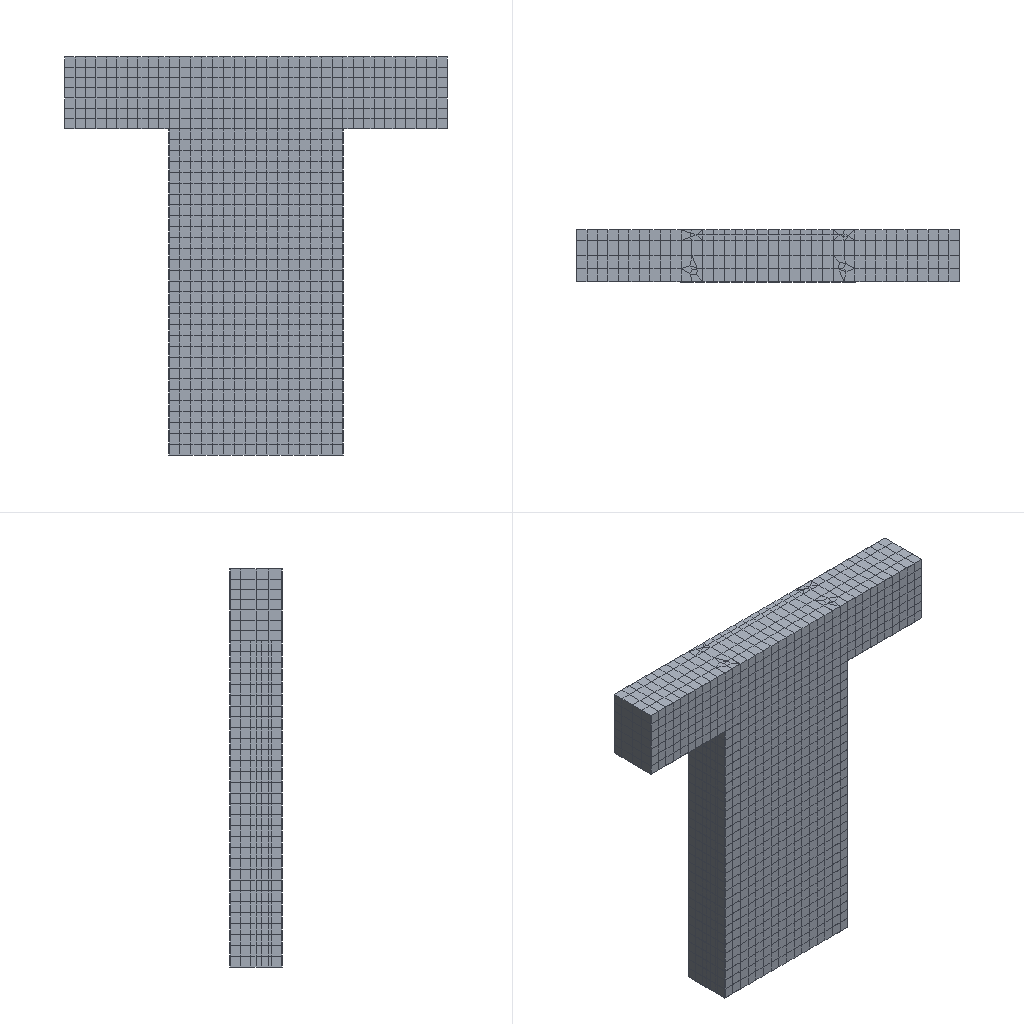Simulation study | abaqus
Set-up summary:
category,name,step,type,value,unit,region
solver,abaqus
solver,version,,,Abaqus/Standard 2020
units,not stated in the deck,,not stated
analysis,deck,,static,static
load_step,Step-1,Step-1,static
load_step,Step-2,Step-2,static
load_step,requested,,,2
mesh,nodes,,,10068
mesh,elements,,,7418
element_type,C3D6,,solid,444
element_type,T3D2,,truss,2018
element_type,C3D8R,,solid,4956
load,load commands in deck,,count,2
bc,support commands in deck,,count,7
material,CON,,in results
material,Q235,,in results
check,setup vs results,,match,"per instance, exact: element labels, types and connectivity; labels of the nodes the elements use; coordinates of those nodes at SINGLE_PRECISION in 1 of 4 instance(s)"
Abaqus input file, long lists of numbers shortened:
*Heading
** Job name: Job-3 Model name: Model-1-Copy-Copy
** Generated by: Abaqus/CAE 2020
*Preprint, echo=NO, model=NO, history=NO, contact=NO
**
** PARTS
**
*Part, name=con
*Node
      1,         489.,          90.,        1500.
      2,        -111.,          90.,        1500.
** (5932 more lines like these left out)
*Element, type=C3D8R
  1,    5, 1585,  129,    1, 1654, 3925, 3903, 1653
  2, 1585, 1586,  130,  129, 3925, 3926, 3904, 3903
** (3814 more lines like these left out)
*Element, type=C3D6
1093,    5,   23,    1,  345,  546,  307
1094, 2438,   27,   28, 4466,  439,  547
** (442 more lines like these left out)
*Nset, nset=Set-12
    1,    2,    3,    4,    5,    6,    7,    8,    9,   10,   11,   12,   13,   14,   15,   16
   17,   18,   19,   20,   21,   22,   23,   24,   25,   26,   27,   28,   29,   30,   31,   32
** (360 more lines like these left out)
*Elset, elset=Set-12
    1,    2,    3,    4,    5,    6,    7,    8,    9,   10,   11,   12,   13,   14,   15,   16
   17,   18,   19,   20,   21,   22,   23,   24,   25,   26,   27,   28,   29,   30,   31,   32
** (249 more lines like these left out)
*Nset, nset=Set-14, generate
    1,  5934,     1
*Elset, elset=Set-14, generate
    1,  4260,     1
** Section: con
*Solid Section, elset=Set-14, material=con
,
*End Part
**
*Part, name=fiber
*Node
      1,         734.,          52.,        1525.
      2,         734.,         115.,        1525.
** (1652 more lines like these left out)
*Element, type=T3D2
1, 2, 1
2,   3, 873
** (2016 more lines like these left out)
*Nset, nset=Set-3, generate
    1,  1654,     1
*Elset, elset=Set-3, generate
    1,  2018,     1
*Nset, nset=nei
    1,    2,    3,    4,    5,    6,    7,    8,    9,   10,   11,   12,   13,   14,   15,   16
   17,   18,   19,   20,   21,   22,   23,   24,   25,   26,   27,   28,   29,   30,   31,   32
** (39 more lines like these left out)
*Elset, elset=nei
    1,    2,    3,    4,    5,    6,    7,    8,    9,   10,   11,   12,   13,   14,   15,   16
   17,   18,   19,   20,   21,   22,   23,   24,   25,   26,   27,   28,   29,   30,   31,   32
** (45 more lines like these left out)
** Section: fiber
*Solid Section, elset=Set-3, material=q235
12.56,
*End Part
**
*Part, name=liang1
*Node
      1,         588.,         140.,        1500.
      2,         588.,         140.,           0.
** (1238 more lines like these left out)
*Element, type=C3D8R
 1,   8, 145, 922, 176,   1,  57, 893, 116
 2, 145, 144, 923, 922,  57,  58, 894, 893
** (568 more lines like these left out)
*Nset, nset=Set-1, generate
    1,  1240,     1
*Elset, elset=Set-1, generate
   1,  570,    1
** Section: liang
*Solid Section, elset=Set-1, material=q235
,
*End Part
**
*Part, name=liang2
*Node
      1,        -112.,         -99.,           0.
      2,        -112.,         -99.,        1500.
** (1238 more lines like these left out)
*Element, type=C3D8R
 1, 174, 893, 922, 173,   1,  57, 114,   4
 2, 893, 894, 923, 922,  57,  58, 113, 114
** (568 more lines like these left out)
*Nset, nset=Set-1, generate
    1,  1240,     1
*Elset, elset=Set-1, generate
   1,  570,    1
** Section: liang
*Solid Section, elset=Set-1, material=q235
,
*End Part
**
**
** ASSEMBLY
**
*Assembly, name=Assembly
**
*Instance, name=con-1, part=con
*End Instance
**
*Instance, name=fiber-1, part=fiber
*End Instance
**
*Instance, name=liang1-1, part=liang1
*End Instance
**
*Instance, name=liang2-1, part=liang2
*End Instance
**
*Node
      1,         189.,          20.,           0.
*Node
      2,         189.,          20.,        1830.
*Nset, nset=Set-15
 1,
*Nset, nset=Set-16
 1,
*Nset, nset=Set-18
 2,
*Nset, nset=insert, instance=fiber-1
    1,    2,    3,    4,    5,    6,    7,    8,    9,   10,   11,   12,   13,   14,   15,   16
   17,   18,   19,   20,   21,   22,   23,   24,   25,   26,   27,   28,   29,   30,   31,   32
** (42 more lines like these left out)
*Nset, nset=m_Set-6, instance=fiber-1
    1,    2,    3,    4,    5,    6,    7,    8,    9,   10,   11,   12,   13,   14,   15,   16
   17,   18,   19,   20,   21,   22,   23,   24,   25,   26,   27,   28,   29,   30,   31,   32
** (40 more lines like these left out)
*Elset, elset=m_Set-6, instance=fiber-1
    1,    2,    3,    4,    5,    6,    7,    8,    9,   10,   11,   12,   13,   14,   15,   16
   17,   18,   19,   20,   21,   22,   23,   24,   25,   26,   27,   28,   29,   30,   31,   32
** (48 more lines like these left out)
*Nset, nset=m_Set-8, instance=fiber-1
    1,    2,    3,    4,    5,    6,    7,    8,    9,   10,   11,   12,   13,   14,   15,   16
   17,   18,   19,   20,   21,   22,   23,   24,   25,   26,   27,   28,   29,   30,   31,   32
** (38 more lines like these left out)
*Elset, elset=m_Set-8, instance=fiber-1
    1,    2,    3,    4,    5,    6,    7,    8,    9,   10,   11,   12,   13,   14,   15,   16
   17,   18,   19,   20,   21,   22,   23,   24,   25,   26,   27,   28,   29,   30,   31,   32
** (45 more lines like these left out)
*Nset, nset=m_Set-10, instance=fiber-1
    1,    2,    3,    4,    5,    6,    7,    8,    9,   10,   11,   12,   13,   14,   15,   16
   17,   18,   19,   20,   21,   22,   23,   24,   25,   26,   27,   28,   29,   30,   31,   32
** (38 more lines like these left out)
*Elset, elset=m_Set-10, instance=fiber-1
    1,    2,    3,    4,    5,    6,    7,    8,    9,   10,   11,   12,   13,   14,   15,   16
   17,   18,   19,   20,   21,   22,   23,   24,   25,   26,   27,   28,   29,   30,   31,   32
** (45 more lines like these left out)
*Nset, nset=m_Set-12, instance=fiber-1
    1,    2,    3,    4,    5,    6,    7,    8,    9,   10,   11,   12,   13,   14,   15,   16
   17,   18,   19,   20,   21,   22,   23,   24,   25,   26,   27,   28,   29,   30,   31,   32
** (91 more lines like these left out)
*Elset, elset=m_Set-12, instance=fiber-1
    1,    2,    3,    4,    5,    6,    7,    8,    9,   10,   11,   12,   13,   14,   15,   16
   17,   18,   19,   20,   21,   22,   23,   24,   25,   26,   27,   28,   29,   30,   31,   32
** (110 more lines like these left out)
*Nset, nset=m_Set-14
 1,
*Nset, nset=m_Set-17
 2,
*Nset, nset=s_Set-6, instance=con-1
    1,    2,    3,    4,    5,    6,    7,    8,    9,   10,   11,   12,   13,   14,   15,   16
   17,   18,   19,   20,   21,   22,   23,   24,   25,   26,   27,   28,   29,   30,   31,   32
** (360 more lines like these left out)
*Elset, elset=s_Set-6, instance=con-1
    1,    2,    3,    4,    5,    6,    7,    8,    9,   10,   11,   12,   13,   14,   15,   16
   17,   18,   19,   20,   21,   22,   23,   24,   25,   26,   27,   28,   29,   30,   31,   32
** (249 more lines like these left out)
*Nset, nset=s_Set-10, instance=con-1, generate
    1,  5934,     1
*Elset, elset=s_Set-10, instance=con-1, generate
    1,  4260,     1
*Nset, nset=s_Set-12, instance=con-1, generate
    1,  5934,     1
*Elset, elset=s_Set-12, instance=con-1, generate
    1,  4260,     1
*Elset, elset=_m_Surf-5_S1, internal, instance=con-1, generate
 3670,  3673,     1
*Elset, elset=_m_Surf-5_S5, internal, instance=con-1
  444,  468,  492,  516,  540,  564,  588,  612,  636,  660,  684,  708,  732,  756,  780,  804
  828,  852,  876,  900,  924,  948,  972,  996, 1020, 1044, 1068, 1092, 2104, 2164, 2200, 2208
** (4 more lines like these left out)
*Elset, elset=_m_Surf-5_S4, internal, instance=con-1
 2193, 2198, 2201, 2206, 2209, 2214, 2217, 2222, 2225, 2230, 2233, 2238, 2241, 2246, 2249, 2254
 2257, 2262, 2265, 2270, 2273, 2278, 2281, 2286, 2289, 2294, 2297, 2302, 2305, 2310, 2313, 2318
** (10 more lines like these left out)
*Elset, elset=_m_Surf-5_S3, internal, instance=con-1
 2197, 2205, 2213, 2221, 2229, 2237, 2245, 2253, 2261, 2269, 2277, 2285, 2293, 2301, 2309, 2317
 2325, 2333, 2341, 2349, 2357, 2365, 2373, 2381, 2389, 2397, 2405, 2413, 2418, 2422, 2426, 2430
** (2 more lines like these left out)
*Elset, elset=_m_Surf-5_S6, internal, instance=con-1
 1396, 1420, 1444, 1468, 1492, 1516, 1540, 1564, 1588, 1612, 1636, 1660, 1684, 1708, 1732, 1756
 1780, 1804, 1828, 1852, 1876, 1900, 1924, 1948, 1972, 1996, 2020, 2044, 2068, 2128, 2197, 2199
** (4 more lines like these left out)
*Surface, type=ELEMENT, name=m_Surf-5
_m_Surf-5_S1, S1
_m_Surf-5_S5, S5
_m_Surf-5_S4, S4
_m_Surf-5_S6, S6
_m_Surf-5_S3, S3
*Elset, elset=_m_Surf-7_S2, internal, instance=liang1-1
   1,   2,   3,   4,   5,   6,   7,   8,   9,  10,  11,  12,  13,  14,  15,  16
  17,  18,  19,  20,  21,  22,  23,  24,  25,  26,  27,  28,  29,  30,  31,  32
** (6 more lines like these left out)
*Elset, elset=_m_Surf-7_S5, internal, instance=liang1-1
 151, 152, 153, 154, 155, 156, 157, 158, 159, 160, 161, 162, 163, 164, 165, 166
 167, 168, 169, 170, 171, 172, 173, 174, 175, 176, 177, 178, 179, 180, 181, 182
** (6 more lines like these left out)
*Elset, elset=_m_Surf-7_S4, internal, instance=liang1-1
  61,  62,  63,  64,  65,  66,  67,  68,  69,  70,  71,  72,  73,  74,  75,  76
  77,  78,  79,  80,  81,  82,  83,  84,  85,  86,  87,  88,  89,  90, 270, 390
*Elset, elset=_m_Surf-7_S6, internal, instance=liang1-1
 241, 361
*Elset, elset=_m_Surf-7_S1, internal, instance=liang1-1
 241, 242, 243, 244, 245, 246, 247, 248, 249, 250, 251, 252, 253, 254, 255, 256
 257, 258, 259, 260, 261, 262, 263, 264, 265, 266, 267, 268, 269, 270, 541, 542
** (2 more lines like these left out)
*Elset, elset=_m_Surf-7_S3, internal, instance=liang1-1, generate
 361,  540,    1
*Surface, type=ELEMENT, name=m_Surf-7
_m_Surf-7_S2, S2
_m_Surf-7_S5, S5
_m_Surf-7_S4, S4
_m_Surf-7_S6, S6
_m_Surf-7_S1, S1
_m_Surf-7_S3, S3
*Elset, elset=_m_Surf-9_S6, internal, instance=con-1
 2194, 2202, 2210, 2218, 2226, 2234, 2242, 2250, 2258, 2266, 2274, 2282, 2290, 2298, 2306, 2314
 2322, 2330, 2338, 2346, 2354, 2362, 2370, 2378, 2386, 2394, 2402, 2410, 2531, 2535, 2539, 2543
** (4 more lines like these left out)
*Elset, elset=_m_Surf-9_S3, internal, instance=con-1
 2199, 2207, 2215, 2223, 2231, 2239, 2247, 2255, 2263, 2271, 2279, 2287, 2295, 2303, 2311, 2319
 2327, 2335, 2343, 2351, 2359, 2367, 2375, 2383, 2391, 2399, 2407, 2415, 2646, 2653, 2660, 2667
*Surface, type=ELEMENT, name=m_Surf-9
_m_Surf-9_S6, S6
_m_Surf-9_S3, S3
*Elset, elset=_m_Surf-11_S6, internal, instance=con-1
 2711, 2719, 2727, 2735, 2743, 2751, 2759, 2767, 2775, 2783, 2791, 2799, 2807, 2815, 2823, 2831
 2839, 2847, 2855, 2863, 2871, 2879, 2887, 2895, 2903, 2911, 2919, 2927, 2935, 2949, 2973, 2974
** (2 more lines like these left out)
*Elset, elset=_m_Surf-11_S3, internal, instance=con-1
 2709, 2717, 2725, 2733, 2741, 2749, 2757, 2765, 2773, 2781, 2789, 2797, 2805, 2813, 2821, 2829
 2837, 2845, 2853, 2861, 2869, 2877, 2885, 2893, 2901, 2909, 2917, 2925, 2933, 2940, 2947, 2954
*Elset, elset=_m_Surf-11_S4, internal, instance=con-1
 1094, 1100, 1106, 1112, 1118, 1124, 1130, 1136, 1142, 1148, 1154, 1160, 1166, 1172, 1178, 1184
 1190, 1196, 1202, 1208, 1214, 1220, 1226, 1232, 1238, 1244, 1250, 1256, 2961, 2968
*Surface, type=ELEMENT, name=m_Surf-11
_m_Surf-11_S6, S6
_m_Surf-11_S3, S3
_m_Surf-11_S4, S4
*Elset, elset=_m_Surf-14_S1, internal, instance=con-1
 3653, 3654, 3655, 3656, 3670, 3671, 3672, 3673
*Elset, elset=_m_Surf-14_S5, internal, instance=con-1
  444,  468,  492,  516,  540,  564,  588,  612,  636,  660,  684,  708,  732,  756,  780,  804
  828,  852,  876,  900,  924,  948,  972,  996, 1020, 1044, 1068, 1092, 2104, 2164, 2200, 2208
** (4 more lines like these left out)
*Elset, elset=_m_Surf-14_S4, internal, instance=con-1
 2193, 2198, 2201, 2206, 2209, 2214, 2217, 2222, 2225, 2230, 2233, 2238, 2241, 2246, 2249, 2254
 2257, 2262, 2265, 2270, 2273, 2278, 2281, 2286, 2289, 2294, 2297, 2302, 2305, 2310, 2313, 2318
** (10 more lines like these left out)
*Elset, elset=_m_Surf-14_S3, internal, instance=con-1
 2197, 2205, 2213, 2221, 2229, 2237, 2245, 2253, 2261, 2269, 2277, 2285, 2293, 2301, 2309, 2317
 2325, 2333, 2341, 2349, 2357, 2365, 2373, 2381, 2389, 2397, 2405, 2413, 2418, 2422, 2426, 2430
** (2 more lines like these left out)
*Elset, elset=_m_Surf-14_S6, internal, instance=con-1
 1396, 1420, 1444, 1468, 1492, 1516, 1540, 1564, 1588, 1612, 1636, 1660, 1684, 1708, 1732, 1756
 1780, 1804, 1828, 1852, 1876, 1900, 1924, 1948, 1972, 1996, 2020, 2044, 2068, 2128, 2197, 2199
** (4 more lines like these left out)
*Surface, type=ELEMENT, name=m_Surf-14
_m_Surf-14_S1, S1
_m_Surf-14_S5, S5
_m_Surf-14_S4, S4
_m_Surf-14_S6, S6
_m_Surf-14_S3, S3
*Elset, elset=_s_Surf-1_S2, internal, instance=con-1, generate
 361,  420,    1
*Surface, type=ELEMENT, name=s_Surf-1
_s_Surf-1_S2, S2
*Elset, elset=_s_Surf-3_S5, internal, instance=con-1
 3001, 3023, 3045, 3067, 3089, 3111, 3133, 3241, 3244, 3283, 3286, 3325, 3328, 3367, 3370, 3409
 3412, 3451, 3454, 3493, 3496, 3535, 3538, 3577, 3580, 3619, 3622, 3878, 3880, 3920, 3922, 3962
** (1 more lines like these left out)
*Elset, elset=_s_Surf-3_S3, internal, instance=con-1
 3002, 3024, 3046, 3068, 3090, 3112, 3134, 3242, 3243, 3245, 3284, 3285, 3287, 3326, 3327, 3329
 3368, 3369, 3371, 3410, 3411, 3413, 3452, 3453, 3455, 3494, 3495, 3497, 3536, 3537, 3539, 3578
** (3 more lines like these left out)
*Elset, elset=_s_Surf-3_S2, internal, instance=con-1, generate
 2105,  2164,     1
*Elset, elset=_s_Surf-3_S4, internal, instance=con-1
 3240, 3282, 3324, 3366, 3408, 3450, 3492, 3534, 3576, 3618, 3882, 3924, 3966, 4008, 4050, 4092
 4134, 4176, 4218, 4260
*Surface, type=ELEMENT, name=s_Surf-3
_s_Surf-3_S5, S5
_s_Surf-3_S3, S3
_s_Surf-3_S2, S2
_s_Surf-3_S4, S4
*Elset, elset=_s_Surf-5_S4, internal, instance=liang2-1
  30,  60,  90, 120, 181, 182, 183, 184, 185, 186, 187, 188, 189, 190, 191, 192
 193, 194, 195, 196, 197, 198, 199, 200, 201, 202, 203, 204, 205, 206, 207, 208
** (1 more lines like these left out)
*Elset, elset=_s_Surf-5_S6, internal, instance=liang2-1
  91, 151, 152, 153, 154, 155, 156, 157, 158, 159, 160, 161, 162, 163, 164, 165
 166, 167, 168, 169, 170, 171, 172, 173, 174, 175, 176, 177, 178, 179, 180, 181
** (3 more lines like these left out)
*Elset, elset=_s_Surf-5_S2, internal, instance=liang2-1
  91,  92,  93,  94,  95,  96,  97,  98,  99, 100, 101, 102, 103, 104, 105, 106
 107, 108, 109, 110, 111, 112, 113, 114, 115, 116, 117, 118, 119, 120, 151, 271
** (8 more lines like these left out)
*Elset, elset=_s_Surf-5_S3, internal, instance=liang2-1
   1,   2,   3,   4,   5,   6,   7,   8,   9,  10,  11,  12,  13,  14,  15,  16
  17,  18,  19,  20,  21,  22,  23,  24,  25,  26,  27,  28,  29,  30,  31,  32
** (4 more lines like these left out)
*Elset, elset=_s_Surf-5_S5, internal, instance=liang2-1
  91,  92,  93,  94,  95,  96,  97,  98,  99, 100, 101, 102, 103, 104, 105, 106
 107, 108, 109, 110, 111, 112, 113, 114, 115, 116, 117, 118, 119, 120, 151, 152
** (8 more lines like these left out)
*Elset, elset=_s_Surf-5_S1, internal, instance=liang2-1
  91,  92,  93,  94,  95,  96,  97,  98,  99, 100, 101, 102, 103, 104, 105, 106
 107, 108, 109, 110, 111, 112, 113, 114, 115, 116, 117, 118, 119, 120, 180, 211
** (6 more lines like these left out)
*Surface, type=ELEMENT, name=s_Surf-5
_s_Surf-5_S4, S4
_s_Surf-5_S6, S6
_s_Surf-5_S2, S2
_s_Surf-5_S3, S3
_s_Surf-5_S5, S5
_s_Surf-5_S1, S1
*Elset, elset=_s_Surf-7_S1, internal, instance=con-1, generate
 3001,  3008,     1
*Elset, elset=_s_Surf-7_S3, internal, instance=con-1
  433,  457,  481,  505,  529,  553,  577,  601,  625,  649,  673,  697,  721,  745,  769,  793
  817,  841,  865,  889,  913,  937,  961,  985, 1009, 1033, 1057, 1081, 1093, 1099, 1105, 1111
** (4 more lines like these left out)
*Elset, elset=_s_Surf-7_S4, internal, instance=con-1
 1095, 1101, 1107, 1113, 1119, 1125, 1131, 1137, 1143, 1149, 1155, 1161, 1167, 1173, 1179, 1185
 1191, 1197, 1203, 1209, 1215, 1221, 1227, 1233, 1239, 1245, 1251, 1257, 1262, 1266, 1270, 1274
** (6 more lines like these left out)
*Elset, elset=_s_Surf-7_S5, internal, instance=con-1
 1095, 1101, 1107, 1113, 1119, 1125, 1131, 1137, 1143, 1149, 1155, 1161, 1167, 1173, 1179, 1185
 1191, 1197, 1203, 1209, 1215, 1221, 1227, 1233, 1239, 1245, 1251, 1257, 1263, 1264, 1267, 1268
** (8 more lines like these left out)
*Elset, elset=_s_Surf-7_S6, internal, instance=con-1
 2707, 2713, 2715, 2721, 2723, 2729, 2731, 2737, 2739, 2745, 2747, 2753, 2755, 2761, 2763, 2769
 2771, 2777, 2779, 2785, 2787, 2793, 2795, 2801, 2803, 2809, 2811, 2817, 2819, 2825, 2827, 2833
** (2 more lines like these left out)
*Surface, type=ELEMENT, name=s_Surf-7
_s_Surf-7_S1, S1
_s_Surf-7_S3, S3
_s_Surf-7_S4, S4
_s_Surf-7_S6, S6
_s_Surf-7_S5, S5
*Elset, elset=_s_Surf-9_S3, internal, instance=liang2-1, generate
 391,  540,    1
*Surface, type=ELEMENT, name=s_Surf-9
_s_Surf-9_S3, S3
*Elset, elset=_s_Surf-11_S3, internal, instance=liang1-1, generate
 391,  540,    1
*Surface, type=ELEMENT, name=s_Surf-11
_s_Surf-11_S3, S3
*Elset, elset=_s_Surf-13_S2, internal, instance=con-1, generate
 361,  420,    1
*Elset, elset=_s_Surf-13_S2, internal, instance=liang1-1
 61,
*Elset, elset=_s_Surf-13_S4, internal, instance=liang1-1
  30,  60, 360, 420, 450, 480, 510, 540
*Elset, elset=_s_Surf-13_S4, internal, instance=liang2-1
 120, 300, 330, 390
*Elset, elset=_s_Surf-13_S1, internal, instance=liang1-1
 120, 150
*Elset, elset=_s_Surf-13_S1, internal, instance=liang2-1
 150, 180
*Elset, elset=_s_Surf-13_S6, internal, instance=liang1-1
 151, 181, 211, 241, 271, 301, 361
*Elset, elset=_s_Surf-13_S6, internal, instance=liang2-1
   1,  31,  61, 211, 241, 331, 391, 421, 451, 481, 511
*Elset, elset=_s_Surf-13_S5, internal, instance=liang1-1
 570,
*Elset, elset=_s_Surf-13_S3, internal, instance=liang2-1
 181, 541
*Surface, type=ELEMENT, name=s_Surf-13
_s_Surf-13_S2, S2
_s_Surf-13_S4, S4
_s_Surf-13_S6, S6
_s_Surf-13_S1, S1
_s_Surf-13_S5, S5
_s_Surf-13_S3, S3
*Elset, elset=_s_Surf-15_S2, internal, instance=con-1
  361,  362,  363,  364,  365,  366,  367,  368,  369,  370,  371,  372,  373,  374,  375,  376
  377,  378,  379,  380,  381,  382,  383,  384,  385,  386,  387,  388,  389,  390,  391,  392
** (6 more lines like these left out)
*Elset, elset=_s_Surf-15_S4, internal, instance=con-1
 3240, 3282, 3324, 3366, 3408, 3450, 3492, 3534, 3576, 3618, 3882, 3924, 3966, 4008, 4050, 4092
 4134, 4176, 4218, 4260
*Elset, elset=_s_Surf-15_S5, internal, instance=con-1
 3241, 3244, 3283, 3286, 3325, 3328, 3367, 3370, 3409, 3412, 3451, 3454, 3493, 3496, 3535, 3538
 3577, 3580, 3619, 3622, 3878, 3880, 3920, 3922, 3962, 3964, 4004, 4006, 4046, 4048, 4088, 4090
** (1 more lines like these left out)
*Elset, elset=_s_Surf-15_S3, internal, instance=con-1
 3242, 3243, 3245, 3284, 3285, 3287, 3326, 3327, 3329, 3368, 3369, 3371, 3410, 3411, 3413, 3452
 3453, 3455, 3494, 3495, 3497, 3536, 3537, 3539, 3578, 3579, 3581, 3620, 3621, 3623, 3877, 3879
** (2 more lines like these left out)
*Surface, type=ELEMENT, name=s_Surf-15
_s_Surf-15_S2, S2
_s_Surf-15_S4, S4
_s_Surf-15_S5, S5
_s_Surf-15_S3, S3
*Elset, elset=_s_Surf-16_S2, internal, instance=con-1
 2105, 2106, 2107, 2108, 2109, 2110, 2111, 2112, 2113, 2114, 2115, 2116, 2117, 2118, 2119, 2120
 2121, 2122, 2123, 2124, 2125, 2126, 2127, 2128, 2129, 2130, 2131, 2132, 2133, 2134, 2135, 2136
** (5 more lines like these left out)
*Elset, elset=_s_Surf-16_S2, internal, instance=liang1-1
 61,
*Elset, elset=_s_Surf-16_S4, internal, instance=liang1-1
  30,  60, 360, 420, 450, 480, 510, 540
*Elset, elset=_s_Surf-16_S4, internal, instance=liang2-1
 120, 300, 330, 390
*Elset, elset=_s_Surf-16_S1, internal, instance=liang1-1
 120, 150
*Elset, elset=_s_Surf-16_S1, internal, instance=liang2-1
 150, 180
*Elset, elset=_s_Surf-16_S6, internal, instance=liang1-1
 151, 181, 211, 241, 271, 301, 361
*Elset, elset=_s_Surf-16_S6, internal, instance=liang2-1
   1,  31,  61, 211, 241, 331, 391, 421, 451, 481, 511
*Elset, elset=_s_Surf-16_S5, internal, instance=liang1-1
 570,
*Elset, elset=_s_Surf-16_S3, internal, instance=liang2-1
 181, 541
*Surface, type=ELEMENT, name=s_Surf-16
_s_Surf-16_S2, S2
_s_Surf-16_S4, S4
_s_Surf-16_S6, S6
_s_Surf-16_S1, S1
_s_Surf-16_S5, S5
_s_Surf-16_S3, S3
*Elset, elset=_s_Surf-17_S3, internal, instance=liang2-1, generate
 391,  540,    1
*Surface, type=ELEMENT, name=s_Surf-17
_s_Surf-17_S3, S3
*Elset, elset=_s_Surf-18_S2, internal, instance=con-1
 2105, 2106, 2107, 2108, 2109, 2110, 2111, 2112, 2113, 2114, 2115, 2116, 2117, 2118, 2119, 2120
 2121, 2122, 2123, 2124, 2125, 2126, 2127, 2128, 2129, 2130, 2131, 2132, 2133, 2134, 2135, 2136
** (5 more lines like these left out)
*Elset, elset=_s_Surf-18_S2, internal, instance=liang1-1
 61,
*Elset, elset=_s_Surf-18_S4, internal, instance=liang1-1
  30,  60, 360, 420, 450, 480, 510, 540
*Elset, elset=_s_Surf-18_S4, internal, instance=liang2-1
 120, 300, 330, 390
*Elset, elset=_s_Surf-18_S1, internal, instance=liang1-1
 120, 150
*Elset, elset=_s_Surf-18_S1, internal, instance=liang2-1
 150, 180
*Elset, elset=_s_Surf-18_S6, internal, instance=liang1-1
 151, 181, 211, 241, 271, 301, 361
*Elset, elset=_s_Surf-18_S6, internal, instance=liang2-1
   1,  31,  61, 211, 241, 331, 391, 421, 451, 481, 511
*Elset, elset=_s_Surf-18_S5, internal, instance=liang1-1
 570,
*Elset, elset=_s_Surf-18_S3, internal, instance=liang2-1
 181, 541
*Surface, type=ELEMENT, name=s_Surf-18
_s_Surf-18_S2, S2
_s_Surf-18_S4, S4
_s_Surf-18_S6, S6
_s_Surf-18_S1, S1
_s_Surf-18_S5, S5
_s_Surf-18_S3, S3
*Elset, elset=_s_Surf-19_S2, internal, instance=con-1
  361,  362,  363,  364,  365,  366,  367,  368,  369,  370,  371,  372,  373,  374,  375,  376
  377,  378,  379,  380,  381,  382,  383,  384,  385,  386,  387,  388,  389,  390,  391,  392
** (6 more lines like these left out)
*Elset, elset=_s_Surf-19_S4, internal, instance=con-1
 3240, 3282, 3324, 3366, 3408, 3450, 3492, 3534, 3576, 3618, 3882, 3924, 3966, 4008, 4050, 4092
 4134, 4176, 4218, 4260
*Elset, elset=_s_Surf-19_S5, internal, instance=con-1
 3241, 3244, 3283, 3286, 3325, 3328, 3367, 3370, 3409, 3412, 3451, 3454, 3493, 3496, 3535, 3538
 3577, 3580, 3619, 3622, 3878, 3880, 3920, 3922, 3962, 3964, 4004, 4006, 4046, 4048, 4088, 4090
** (1 more lines like these left out)
*Elset, elset=_s_Surf-19_S3, internal, instance=con-1
 3242, 3243, 3245, 3284, 3285, 3287, 3326, 3327, 3329, 3368, 3369, 3371, 3410, 3411, 3413, 3452
 3453, 3455, 3494, 3495, 3497, 3536, 3537, 3539, 3578, 3579, 3581, 3620, 3621, 3623, 3877, 3879
** (2 more lines like these left out)
*Surface, type=ELEMENT, name=s_Surf-19
_s_Surf-19_S2, S2
_s_Surf-19_S4, S4
_s_Surf-19_S5, S5
_s_Surf-19_S3, S3
*Elset, elset=_s_Surf-20_S2, internal, instance=con-1
 2105, 2106, 2107, 2108, 2109, 2110, 2111, 2112, 2113, 2114, 2115, 2116, 2117, 2118, 2119, 2120
 2121, 2122, 2123, 2124, 2125, 2126, 2127, 2128, 2129, 2130, 2131, 2132, 2133, 2134, 2135, 2136
** (5 more lines like these left out)
*Surface, type=ELEMENT, name=s_Surf-20
_s_Surf-20_S2, S2
*Elset, elset=_s_Surf-21_S2, internal, instance=con-1
 2105, 2106, 2107, 2108, 2109, 2110, 2111, 2112, 2113, 2114, 2115, 2116, 2117, 2118, 2119, 2120
 2121, 2122, 2123, 2124, 2125, 2126, 2127, 2128, 2129, 2130, 2131, 2132, 2133, 2134, 2135, 2136
** (5 more lines like these left out)
*Elset, elset=_s_Surf-21_S2, internal, instance=liang1-1
 61,
*Elset, elset=_s_Surf-21_S4, internal, instance=liang1-1
  30,  60, 360, 420, 450, 480, 510, 540
*Elset, elset=_s_Surf-21_S4, internal, instance=liang2-1
 120, 300, 330, 390
*Elset, elset=_s_Surf-21_S1, internal, instance=liang1-1
 120, 150
*Elset, elset=_s_Surf-21_S1, internal, instance=liang2-1
 150, 180
*Elset, elset=_s_Surf-21_S6, internal, instance=liang1-1
 151, 181, 211, 241, 271, 301, 361
*Elset, elset=_s_Surf-21_S6, internal, instance=liang2-1
   1,  31,  61, 211, 241, 331, 391, 421, 451, 481, 511
*Elset, elset=_s_Surf-21_S5, internal, instance=liang1-1
 570,
*Elset, elset=_s_Surf-21_S3, internal, instance=liang2-1
 181, 541
*Surface, type=ELEMENT, name=s_Surf-21
_s_Surf-21_S2, S2
_s_Surf-21_S4, S4
_s_Surf-21_S6, S6
_s_Surf-21_S1, S1
_s_Surf-21_S5, S5
_s_Surf-21_S3, S3
*Elset, elset=_s_Surf-22_S2, internal, instance=con-1
  361,  362,  363,  364,  365,  366,  367,  368,  369,  370,  371,  372,  373,  374,  375,  376
  377,  378,  379,  380,  381,  382,  383,  384,  385,  386,  387,  388,  389,  390,  391,  392
** (6 more lines like these left out)
*Elset, elset=_s_Surf-22_S4, internal, instance=con-1
 3240, 3282, 3324, 3366, 3408, 3450, 3492, 3534, 3576, 3618, 3882, 3924, 3966, 4008, 4050, 4092
 4134, 4176, 4218, 4260
*Elset, elset=_s_Surf-22_S5, internal, instance=con-1
 3241, 3244, 3283, 3286, 3325, 3328, 3367, 3370, 3409, 3412, 3451, 3454, 3493, 3496, 3535, 3538
 3577, 3580, 3619, 3622, 3878, 3880, 3920, 3922, 3962, 3964, 4004, 4006, 4046, 4048, 4088, 4090
** (1 more lines like these left out)
*Elset, elset=_s_Surf-22_S3, internal, instance=con-1
 3242, 3243, 3245, 3284, 3285, 3287, 3326, 3327, 3329, 3368, 3369, 3371, 3410, 3411, 3413, 3452
 3453, 3455, 3494, 3495, 3497, 3536, 3537, 3539, 3578, 3579, 3581, 3620, 3621, 3623, 3877, 3879
** (2 more lines like these left out)
*Surface, type=ELEMENT, name=s_Surf-22
_s_Surf-22_S2, S2
_s_Surf-22_S4, S4
_s_Surf-22_S5, S5
_s_Surf-22_S3, S3
** Constraint: Constraint-4
*Tie, name=Constraint-4, adjust=yes
s_Surf-11, m_Surf-11
** Constraint: Constraint-dong
*Coupling, constraint name=Constraint-dong, ref node=m_Set-14, surface=s_Surf-21
*Kinematic
** Constraint: Constraint-fix
*Coupling, constraint name=Constraint-fix, ref node=m_Set-17, surface=s_Surf-22
*Kinematic
** Constraint: Constraint-liang
*Tie, name=Constraint-liang, adjust=yes
m_Surf-9, s_Surf-17
** Constraint: Constraint-nei
*Embedded Element, host elset=s_Set-12
m_Set-12
*End Assembly
*Amplitude, name=Amp-1
             0.,              0.,              1.,              1.
*Amplitude, name=Amp-load
             0.,              0.,             0.5,             0.1,              1.,            -0.1,             1.5,              0.
             2.,             0.4,             2.5,            -0.4,              3.,              0.,             3.5,             0.6
             4.,            -0.6,             4.5,              0.,              5.,             0.9,             5.5,            -0.9
             6.,              0.,             6.5,              1.,              7.,             -1.,             7.5,              0.
             8.,             1.3,             8.5,            -1.3,              9.,              0.,             9.5,             1.6
            10.,            -1.6,            10.5,              0.,             11.,             1.9,            11.5,            -1.9
            12.,              0.,            12.5,             2.4,             13.,            -2.4,            13.5,              0.
            14.,             2.8,            14.5,            -2.8,             15.,              0.,            15.5,             3.2
            16.,            -3.2,            16.5,              0.,             17.,             3.6,            17.5,            -3.6
            18.,              0.,            18.5,              4.,             19.,             -4.,            19.5,              0.
            20.,             4.4,            20.5,            -4.4,             21.,              0.,            21.5,             4.8
            22.,            -4.8,            22.5,              0.,             23.,             5.2,            23.5,            -5.2
            24.,              0.,            24.5,             5.6,             25.,            -5.6,            25.5,              0.
            26.,              6.,            26.5,             -6.,             27.,              0.,            27.5,             6.5
            28.,            -6.5,            28.5,              0.,             29.,              7.,            29.5,             -7.
            30.,              0.,            30.5,             7.5,             31.,            -7.5,            31.5,              0.
            32.,              8.,            32.5,             -8.,             33.,              0.,            33.5,             8.5
            34.,            -8.5,            34.5,              0.,             35.,              9.,            35.5,             -9.
            36.,              0.,            36.5,             9.6,             37.,            -9.6,            37.5,              0.
            38.,            10.2,            38.5,           -10.2,             39.,              0.,            39.5,            10.8
            40.,           -10.8,            40.5,              0.,             41.,            11.4,            41.5,           -11.4
            42.,              0.,            42.5,             12.,             43.,            -12.,            43.5,              0.
            44.,            12.7,            44.5,           -12.7,             45.,              0.,            45.5,            13.4
            46.,           -13.4,            46.5,              0.,             47.,            14.1,            47.5,           -14.1
            48.,              0.,            48.5,            14.9,             49.,           -14.9,            49.5,              0.
            50.,            15.7,            50.5,           -15.7,             51.,              0.,            51.5,            16.5
            52.,           -16.5,            52.5,              0.
**
** MATERIALS
**
*Material, name=con
*Elastic
2260., 0.2
*Concrete Damaged Plasticity
45.,     0.1,    1.16,  0.6667, 0.00075
*Concrete Compression Hardening
  2.669,         0.
  3.127, 0.001499
  3.503, 0.001799
 3.659, 0.001949
  3.795, 0.002099
 3.909, 0.002249
  4.003, 0.002399
 4.076,  0.002549
  4.128, 0.002699
 4.16, 0.002849
    4.17, 0.002999
  4.087,  0.003299
  4.003, 0.003599
  3.92, 0.003899
  3.836, 0.004199
   3.753, 0.004499
  3.67, 0.004799
*Concrete Tension Stiffening
   0.1984,         0.
   0.2325, 0.0015
   0.2604, 0.0018
 0.272, 0.00195
   0.2821, 0.0021
 0.2906, 0.00225
   0.2976, 0.0024
 0.303, 0.00255
   0.3069, 0.0027
 0.3092, 0.00285
     0.31, 0.003
   0.3038, 0.0033
   0.2976, 0.0036
   0.2914, 0.0039
   0.2852, 0.0042
    0.279, 0.0045
   0.2728, 0.0048
*Concrete Compression Damage
        0.,         0.
 0.0395, 0.001499
 0.07207, 0.001799
 0.08879, 0.001949
   0.1058, 0.002099
  0.1232, 0.002249
    0.1409, 0.002399
  0.159,  0.002549
  0.1775, 0.002699
  0.1964, 0.002849
  0.2158, 0.002999
  0.2598,  0.003299
  0.2985, 0.003599
  0.3331, 0.003899
  0.3643, 0.004199
  0.3925, 0.004499
  0.4184, 0.004799
*Concrete Tension Damage
       0.,         0.
 0.7381, 0.0015
 0.747, 0.0018
 0.7516, 0.00195
 0.7562, 0.0021
 0.7609, 0.00225
 0.7658, 0.0024
 0.7707, 0.00255
 0.7757, 0.0027
 0.7809, 0.00285
 0.7862, 0.003
 0.7982, 0.0033
 0.8087, 0.0036
 0.8182, 0.0039
 0.8267, 0.0042
 0.8344, 0.0045
  0.8414, 0.0048
*Material, name=q235
*Elastic
124500., 0.25
*Plastic
 50.,      0.
 80.,  0.0001
100.,  0.0005
180.,   0.001
250.,  0.0016
 80.,  0.0024
 40.,  0.0028
 10., 0.00323
**
** INTERACTION PROPERTIES
**
*Surface Interaction, name=IntProp-1
1.,
*Friction, slip tolerance=0.005
 0.2,
*Surface Behavior, pressure-overclosure=HARD
**
** INTERACTIONS
**
** Interaction: Int-1
*Contact Pair, interaction=IntProp-1, type=SURFACE TO SURFACE, adjust=1.
s_Surf-5, m_Surf-14
** Interaction: Int-2
*Contact Pair, interaction=IntProp-1, type=SURFACE TO SURFACE, adjust=1.
m_Surf-7, s_Surf-7
** ----------------------------------------------------------------
**
** STEP: Step-1
**
*Step, name=Step-1, nlgeom=NO, inc=1000
*Static
0.01, 1., 1e-05, 1.
**
** BOUNDARY CONDITIONS
**
** Name: [REDACTED] : Symmetric / antisymmetric / fully fixed
*Boundary
Set-18, ENCASTRE
**
** LOADS
**
** Name: Load-1   Type: Concentrated force
*Cload, amplitude=Amp-load
Set-16, 3, 259200.
**
** OUTPUT REQUESTS
**
*Restart, write, frequency=0
**
** FIELD OUTPUT: F-Output-1
**
*Output, field, variable=PRESELECT
*Output, history, frequency=0
*End Step
** ----------------------------------------------------------------
**
** STEP: Step-2
**
*Step, name=Step-2, nlgeom=NO, inc=5000
*Static
0.1, 54.5, 0.0001, 54.5
**
** BOUNDARY CONDITIONS
**
** Name: [REDACTED] : Displacement/rotation angle
*Boundary, amplitude=Amp-load
Set-15, 1, 1, 1.
Set-15, 2, 2
Set-15, 3, 3
Set-15, 4, 4
Set-15, 5, 5
Set-15, 6, 6
**
** OUTPUT REQUESTS
**
*Restart, write, frequency=0
**
** FIELD OUTPUT: F-Output-1
**
*Output, field
*Node Output
CF, RF, RM, RT, U, V
*Element Output, directions=YES
DAMAGEC, DAMAGET, E, LE, MISES, MISESMAX, MISESONLY, P, PE, PEEQ, PEEQMAX, PEEQT, PEMAG, S, SDEG, SF
SSAVG
*Contact Output
CDISP, CSTRESS
**
** HISTORY OUTPUT: H-Output-1
**
*Output, history
*Node Output, nset=Set-15
RF1, U1
*End Step
Results summary:
result,step,,completed,increments=11 time=1.0/1.0
result,step,,partial,increments=269 time=25.98/54.5
result,analysis,,,static
result,last_loadstep,,,2
result,primary field,,,U
result,reaction total,,FX,0.0,model units
result,reaction total,,FY,-0.000671,model units
result,reaction total,,FZ,25919.984,model units